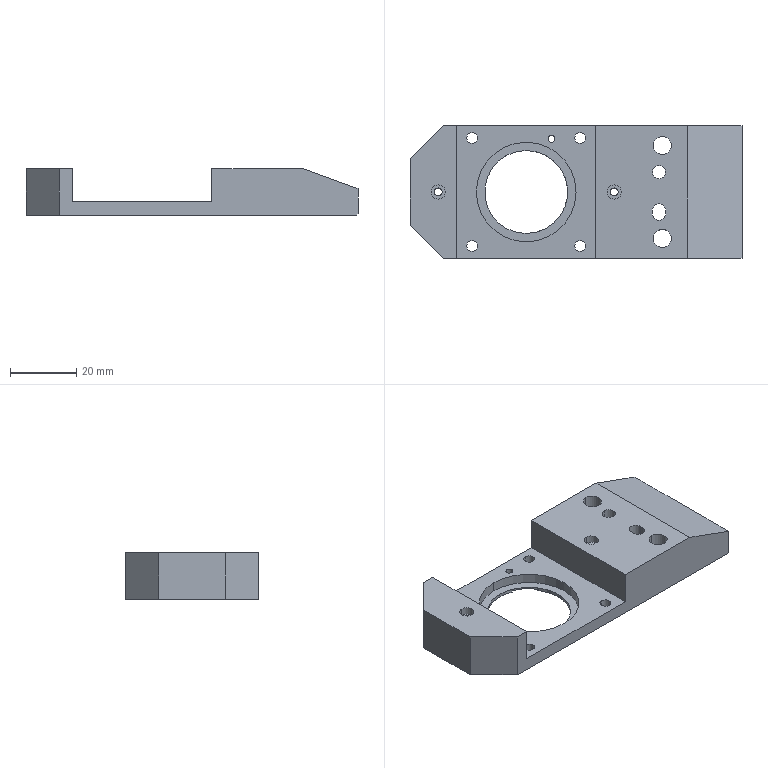NC program | NX | posted with a generic post | part box 100 x 40 x 14 mm
Whole program:
N10 G17 G21 G94 G90
(FLOOR_WALL_COPY_COPY , TOOL : D50R0.8)
N12 T03 M6
N14 G54
N16 G17 G0 G90 X-78.25 Y0. S1000 M3
N18 G43 Z30. H3
N20 Z8.707
N22 G94 G1 Z5.707 F1500.
N24 X-75.25
N26 X74.75
N28 X77.75
N30 Z8.707
N32 G0 Z30.
N34 X-78.25
N36 Z8.415
N38 G1 Z5.415
N40 X-75.25
N42 X74.75
N44 X77.75
N46 Z8.415
N48 G0 Z30.
N50 X-78.25
N52 Z8.122
N54 G1 Z5.122
N56 X-75.25
N58 X74.75
N60 X77.75
N62 Z8.122
N64 G0 Z30.
N66 X-78.25
N68 Z7.83
N70 G1 Z4.83
N72 X-75.25
N74 X74.75
N76 X77.75
N78 Z7.83
N80 G0 Z30.
N82 X-78.25
N84 Z7.537
N86 G1 Z4.537
N88 X-75.25
N90 X74.75
N92 X77.75
N94 Z7.537
N96 G0 Z30.
N98 X-78.25
N100 Z7.245
N102 G1 Z4.245
N104 X-75.25
N106 X74.75
N108 X77.75
N110 Z7.245
N112 G0 Z30.
N114 X-78.25
N116 Z6.952
N118 G1 Z3.952
N120 X-75.25
N122 X74.75
N124 X77.75
N126 Z6.952
N128 G0 Z30.
N130 X-78.25
N132 Z6.66
N134 G1 Z3.66
N136 X-75.25
N138 X74.75
N140 X77.75
N142 Z6.66
N144 G0 Z30.
N146 X-78.25
N148 Z6.367
N150 G1 Z3.367
N152 X-75.25
N154 X74.75
N156 X77.75
N158 Z6.367
N160 G0 Z30.
N162 X-78.25
N164 Z6.075
N166 G1 Z3.075
N168 X-75.25
N170 X74.75
N172 X77.75
N174 Z6.075
N176 G0 Z30.
N178 X-78.25
N180 Z5.782
N182 G1 Z2.782
N184 X-75.25
N186 X74.75
N188 X77.75
N190 Z5.782
N192 G0 Z30.
N194 X-78.25
N196 Z5.49
N198 G1 Z2.49
N200 X-75.25
N202 X74.75
N204 X77.75
N206 Z5.49
N208 G0 Z30.
N210 X-78.25
N212 Z5.197
N214 G1 Z2.197
N216 X-75.25
N218 X74.75
N220 X77.75
N222 Z5.197
N224 G0 Z30.
N226 X-78.25
N228 Z4.905
N230 G1 Z1.905
N232 X-75.25
N234 X74.75
N236 X77.75
N238 Z4.905
N240 G0 Z30.
N242 X-78.25
N244 Z4.612
N246 G1 Z1.612
N248 X-75.25
N250 X74.75
N252 X77.75
N254 Z4.612
N256 G0 Z30.
N258 X-78.25
N260 Z4.32
N262 G1 Z1.32
N264 X-75.25
N266 X74.75
N268 X77.75
N270 Z4.32
N272 G0 Z30.
N274 X-78.25
N276 Z4.027
N278 G1 Z1.027
N280 X-75.25
N282 X74.75
N284 X77.75
N286 Z4.027
N288 G0 Z30.
N290 X-78.25
N292 Z3.735
N294 G1 Z0.735
N296 X-75.25
N298 X74.75
N300 X77.75
N302 Z3.735
N304 G0 Z30.
N306 X-78.25
N308 Z3.442
N310 G1 Z0.442
N312 X-75.25
N314 X74.75
N316 X77.75
N318 Z3.442
N320 G0 Z30.
N322 X-78.25
N324 Z3.15
N326 G1 Z0.15
N328 X-75.25
N330 X74.75
N332 X77.75
N334 Z3.15
N336 G0 Z30.
(FLOOR_WALL_COPY_COPY_1 , TOOL : D50R0.8)
N338 X-78.25 S1500
N340 Z3.
N342 G1 Z0. F1000.
N344 X-75.25
N346 X74.75
N348 X77.75
N350 Z3.
N352 G0 Z30.
N354 M5
(HOLE_MILLING_1 , TOOL : D6)
N356 T06 M6
N358 G54
N360 G17 G0 G90 X-26.25 Y14. S4000 M3
N362 G43 Z30. H6
N364 Z0.5
N366 G94 G3 X-27.225 Y14.975 R0.975 F1800.
N368 X-28.2 Y14. R0.975
N370 X-28.2 Y14. Z0.4 I1.95 J0.
N372 X-28.2 Y14. Z0.3 I1.95 J0.
N374 X-28.2 Y14. Z0.2 I1.95 J0.
N376 X-28.2 Y14. Z0.1 I1.95 J0.
N378 X-28.2 Y14. Z0. I1.95 J0.
N380 X-28.2 Y14. Z-0.1 I1.95 J0.
N382 X-28.2 Y14. Z-0.2 I1.95 J0.
N384 X-28.2 Y14. Z-0.3 I1.95 J0.
N386 X-28.2 Y14. Z-0.4 I1.95 J0.
N388 X-28.2 Y14. Z-0.5 I1.95 J0.
N390 X-28.2 Y14. Z-0.6 I1.95 J0.
N392 X-28.2 Y14. Z-0.7 I1.95 J0.
N394 X-28.2 Y14. Z-0.8 I1.95 J0.
N396 X-28.2 Y14. Z-0.9 I1.95 J0.
N398 X-28.2 Y14. Z-1. I1.95 J0.
N400 X-28.2 Y14. Z-1.1 I1.95 J0.
N402 X-28.2 Y14. Z-1.2 I1.95 J0.
N404 X-28.2 Y14. Z-1.3 I1.95 J0.
N406 X-28.2 Y14. Z-1.4 I1.95 J0.
N408 X-28.2 Y14. Z-1.5 I1.95 J0.
N410 X-28.2 Y14. Z-1.6 I1.95 J0.
N412 X-28.2 Y14. Z-1.7 I1.95 J0.
N414 X-28.2 Y14. Z-1.8 I1.95 J0.
N416 X-28.2 Y14. Z-1.9 I1.95 J0.
N418 X-28.2 Y14. Z-2. I1.95 J0.
N420 X-28.2 Y14. Z-2.1 I1.95 J0.
N422 X-28.2 Y14. Z-2.2 I1.95 J0.
N424 X-28.2 Y14. Z-2.3 I1.95 J0.
N426 X-28.2 Y14. Z-2.4 I1.95 J0.
N428 X-28.2 Y14. Z-2.5 I1.95 J0.
N430 X-28.2 Y14. Z-2.6 I1.95 J0.
N432 X-28.2 Y14. Z-2.7 I1.95 J0.
N434 X-28.2 Y14. Z-2.8 I1.95 J0.
N436 X-28.2 Y14. Z-2.9 I1.95 J0.
N438 X-28.2 Y14. Z-3. I1.95 J0.
N440 X-28.2 Y14. Z-3.1 I1.95 J0.
N442 X-28.2 Y14. Z-3.2 I1.95 J0.
N444 X-28.2 Y14. Z-3.3 I1.95 J0.
N446 X-28.2 Y14. Z-3.4 I1.95 J0.
N448 X-28.2 Y14. Z-3.5 I1.95 J0.
N450 X-28.2 Y14. Z-3.6 I1.95 J0.
N452 X-28.2 Y14. Z-3.7 I1.95 J0.
N454 X-28.2 Y14. Z-3.8 I1.95 J0.
N456 X-28.2 Y14. Z-3.9 I1.95 J0.
N458 X-28.2 Y14. Z-4. I1.95 J0.
N460 X-28.2 Y14. Z-4.1 I1.95 J0.
N462 X-28.2 Y14. Z-4.2 I1.95 J0.
N464 X-28.2 Y14. Z-4.3 I1.95 J0.
N466 X-28.2 Y14. Z-4.4 I1.95 J0.
N468 X-28.2 Y14. Z-4.5 I1.95 J0.
N470 X-28.2 Y14. Z-4.6 I1.95 J0.
N472 X-28.2 Y14. Z-4.7 I1.95 J0.
N474 X-28.2 Y14. Z-4.8 I1.95 J0.
N476 X-28.2 Y14. Z-4.9 I1.95 J0.
N478 X-28.2 Y14. Z-5. I1.95 J0.
N480 X-28.2 Y14. Z-5.1 I1.95 J0.
N482 X-28.2 Y14. Z-5.2 I1.95 J0.
N484 X-28.2 Y14. Z-5.3 I1.95 J0.
N486 X-28.2 Y14. Z-5.4 I1.95 J0.
N488 X-28.2 Y14. Z-5.5 I1.95 J0.
N490 X-28.2 Y14. Z-5.6 I1.95 J0.
N492 X-28.2 Y14. Z-5.7 I1.95 J0.
N494 X-26.25 Y12.05 R1.95
N496 X-28.2 Y14. R-1.95
N498 X-27.225 Y13.025 R0.975
N500 X-26.25 Y14. R0.975
N502 G0 Z30.
N504 Y-14.
N506 Z0.5
N508 G3 X-27.225 Y-13.025 R0.975
N510 X-28.2 Y-14. R0.975
N512 X-28.2 Y-14. Z0.4 I1.95 J0.
N514 X-28.2 Y-14. Z0.3 I1.95 J0.
N516 X-28.2 Y-14. Z0.2 I1.95 J0.
N518 X-28.2 Y-14. Z0.1 I1.95 J0.
N520 X-28.2 Y-14. Z0. I1.95 J0.
N522 X-28.2 Y-14. Z-0.1 I1.95 J0.
N524 X-28.2 Y-14. Z-0.2 I1.95 J0.
N526 X-28.2 Y-14. Z-0.3 I1.95 J0.
N528 X-28.2 Y-14. Z-0.4 I1.95 J0.
N530 X-28.2 Y-14. Z-0.5 I1.95 J0.
N532 X-28.2 Y-14. Z-0.6 I1.95 J0.
N534 X-28.2 Y-14. Z-0.7 I1.95 J0.
N536 X-28.2 Y-14. Z-0.8 I1.95 J0.
N538 X-28.2 Y-14. Z-0.9 I1.95 J0.
N540 X-28.2 Y-14. Z-1. I1.95 J0.
N542 X-28.2 Y-14. Z-1.1 I1.95 J0.
N544 X-28.2 Y-14. Z-1.2 I1.95 J0.
N546 X-28.2 Y-14. Z-1.3 I1.95 J0.
N548 X-28.2 Y-14. Z-1.4 I1.95 J0.
N550 X-28.2 Y-14. Z-1.5 I1.95 J0.
N552 X-28.2 Y-14. Z-1.6 I1.95 J0.
N554 X-28.2 Y-14. Z-1.7 I1.95 J0.
N556 X-28.2 Y-14. Z-1.8 I1.95 J0.
N558 X-28.2 Y-14. Z-1.9 I1.95 J0.
N560 X-28.2 Y-14. Z-2. I1.95 J0.
N562 X-28.2 Y-14. Z-2.1 I1.95 J0.
N564 X-28.2 Y-14. Z-2.2 I1.95 J0.
N566 X-28.2 Y-14. Z-2.3 I1.95 J0.
N568 X-28.2 Y-14. Z-2.4 I1.95 J0.
N570 X-28.2 Y-14. Z-2.5 I1.95 J0.
N572 X-28.2 Y-14. Z-2.6 I1.95 J0.
N574 X-28.2 Y-14. Z-2.7 I1.95 J0.
N576 X-28.2 Y-14. Z-2.8 I1.95 J0.
N578 X-28.2 Y-14. Z-2.9 I1.95 J0.
N580 X-28.2 Y-14. Z-3. I1.95 J0.
N582 X-28.2 Y-14. Z-3.1 I1.95 J0.
N584 X-28.2 Y-14. Z-3.2 I1.95 J0.
N586 X-28.2 Y-14. Z-3.3 I1.95 J0.
N588 X-28.2 Y-14. Z-3.4 I1.95 J0.
N590 X-28.2 Y-14. Z-3.5 I1.95 J0.
N592 X-28.2 Y-14. Z-3.6 I1.95 J0.
N594 X-28.2 Y-14. Z-3.7 I1.95 J0.
N596 X-28.2 Y-14. Z-3.8 I1.95 J0.
N598 X-28.2 Y-14. Z-3.9 I1.95 J0.
N600 X-28.2 Y-14. Z-4. I1.95 J0.
N602 X-28.2 Y-14. Z-4.1 I1.95 J0.
N604 X-28.2 Y-14. Z-4.2 I1.95 J0.
N606 X-28.2 Y-14. Z-4.3 I1.95 J0.
N608 X-28.2 Y-14. Z-4.4 I1.95 J0.
N610 X-28.2 Y-14. Z-4.5 I1.95 J0.
N612 X-28.2 Y-14. Z-4.6 I1.95 J0.
N614 X-28.2 Y-14. Z-4.7 I1.95 J0.
N616 X-28.2 Y-14. Z-4.8 I1.95 J0.
N618 X-28.2 Y-14. Z-4.9 I1.95 J0.
N620 X-28.2 Y-14. Z-5. I1.95 J0.
N622 X-28.2 Y-14. Z-5.1 I1.95 J0.
N624 X-28.2 Y-14. Z-5.2 I1.95 J0.
N626 X-28.2 Y-14. Z-5.3 I1.95 J0.
N628 X-28.2 Y-14. Z-5.4 I1.95 J0.
N630 X-28.2 Y-14. Z-5.5 I1.95 J0.
N632 X-28.2 Y-14. Z-5.6 I1.95 J0.
N634 X-28.2 Y-14. Z-5.7 I1.95 J0.
N636 X-26.25 Y-15.95 R1.95
N638 X-28.2 Y-14. R-1.95
N640 X-27.225 Y-14.975 R0.975
N642 X-26.25 Y-14. R0.975
N644 G0 Z30.
N646 X-11.75 Y0.
N648 Z0.5
N650 G3 X-11.975 Y0.225 R0.225
N652 X-12.2 Y0. R0.225
N654 X-12.2 Y0. Z0.4 I0.45 J0.
N656 X-12.2 Y0. Z0.3 I0.45 J0.
N658 X-12.2 Y0. Z0.2 I0.45 J0.
N660 X-12.2 Y0. Z0.1 I0.45 J0.
N662 X-12.2 Y0. Z0. I0.45 J0.
N664 X-12.2 Y0. Z-0.1 I0.45 J0.
N666 X-12.2 Y0. Z-0.2 I0.45 J0.
N668 X-12.2 Y0. Z-0.3 I0.45 J0.
N670 X-12.2 Y0. Z-0.4 I0.45 J0.
N672 X-12.2 Y0. Z-0.5 I0.45 J0.
N674 X-12.2 Y0. Z-0.6 I0.45 J0.
N676 X-12.2 Y0. Z-0.7 I0.45 J0.
N678 X-12.2 Y0. Z-0.8 I0.45 J0.
N680 X-12.2 Y0. Z-0.9 I0.45 J0.
N682 X-12.2 Y0. Z-1. I0.45 J0.
N684 X-12.2 Y0. Z-1.1 I0.45 J0.
N686 X-12.2 Y0. Z-1.2 I0.45 J0.
N688 X-12.2 Y0. Z-1.3 I0.45 J0.
N690 X-12.2 Y0. Z-1.4 I0.45 J0.
N692 X-12.2 Y0. Z-1.5 I0.45 J0.
N694 X-12.2 Y0. Z-1.6 I0.45 J0.
N696 X-12.2 Y0. Z-1.7 I0.45 J0.
N698 X-12.2 Y0. Z-1.8 I0.45 J0.
N700 X-12.2 Y0. Z-1.9 I0.45 J0.
N702 X-12.2 Y0. Z-2. I0.45 J0.
N704 X-12.2 Y0. Z-2.1 I0.45 J0.
N706 X-12.2 Y0. Z-2.2 I0.45 J0.
N708 X-12.2 Y0. Z-2.3 I0.45 J0.
N710 X-12.2 Y0. Z-2.4 I0.45 J0.
N712 X-12.2 Y0. Z-2.5 I0.45 J0.
N714 X-12.2 Y0. Z-2.6 I0.45 J0.
N716 X-12.2 Y0. Z-2.7 I0.45 J0.
N718 X-12.2 Y0. Z-2.8 I0.45 J0.
N720 X-12.2 Y0. Z-2.9 I0.45 J0.
N722 X-12.2 Y0. Z-3. I0.45 J0.
N724 X-12.2 Y0. Z-3.1 I0.45 J0.
N726 X-12.2 Y0. Z-3.2 I0.45 J0.
N728 X-12.2 Y0. Z-3.3 I0.45 J0.
N730 X-12.2 Y0. Z-3.4 I0.45 J0.
N732 X-12.2 Y0. Z-3.5 I0.45 J0.
N734 X-12.2 Y0. Z-3.6 I0.45 J0.
N736 X-12.2 Y0. Z-3.7 I0.45 J0.
N738 X-12.2 Y0. Z-3.8 I0.45 J0.
N740 X-12.2 Y0. Z-3.9 I0.45 J0.
N742 X-12.2 Y0. Z-4. I0.45 J0.
N744 X-12.2 Y0. Z-4.1 I0.45 J0.
N746 X-12.2 Y0. Z-4.2 I0.45 J0.
N748 X-12.2 Y0. Z-4.3 I0.45 J0.
N750 X-12.2 Y0. Z-4.4 I0.45 J0.
N752 X-12.2 Y0. Z-4.5 I0.45 J0.
N754 X-12.2 Y0. Z-4.6 I0.45 J0.
N756 X-12.2 Y0. Z-4.7 I0.45 J0.
N758 X-12.2 Y0. Z-4.8 I0.45 J0.
N760 X-12.2 Y0. Z-4.9 I0.45 J0.
N762 X-12.2 Y0. Z-5. I0.45 J0.
N764 X-12.2 Y0. Z-5.1 I0.45 J0.
N766 X-12.2 Y0. Z-5.2 I0.45 J0.
N768 X-12.2 Y0. Z-5.3 I0.45 J0.
N770 X-12.2 Y0. Z-5.4 I0.45 J0.
N772 X-12.2 Y0. Z-5.5 I0.45 J0.
N774 X-12.2 Y0. Z-5.6 I0.45 J0.
N776 X-12.2 Y0. Z-5.7 I0.45 J0.
N778 X-12.2 Y0. Z-5.8 I0.45 J0.
N780 X-12.2 Y0. Z-5.9 I0.45 J0.
N782 X-12.2 Y0. Z-6. I0.45 J0.
N784 X-11.75 Y-0.45 R0.45
N786 X-12.2 Y0. R-0.45
N788 X-11.975 Y-0.225 R0.225
N790 X-11.75 Y0. R0.225
N792 G0 Z30.
N794 X41.25
N796 Z0.5
N798 G3 X41.025 Y0.225 R0.225
N800 X40.8 Y0. R0.225
N802 X40.8 Y0. Z0.4 I0.45 J0.
N804 X40.8 Y0. Z0.3 I0.45 J0.
N806 X40.8 Y0. Z0.2 I0.45 J0.
N808 X40.8 Y0. Z0.1 I0.45 J0.
N810 X40.8 Y0. Z0. I0.45 J0.
N812 X40.8 Y0. Z-0.1 I0.45 J0.
N814 X40.8 Y0. Z-0.2 I0.45 J0.
N816 X40.8 Y0. Z-0.3 I0.45 J0.
N818 X40.8 Y0. Z-0.4 I0.45 J0.
N820 X40.8 Y0. Z-0.5 I0.45 J0.
N822 X40.8 Y0. Z-0.6 I0.45 J0.
N824 X40.8 Y0. Z-0.7 I0.45 J0.
N826 X40.8 Y0. Z-0.8 I0.45 J0.
N828 X40.8 Y0. Z-0.9 I0.45 J0.
N830 X40.8 Y0. Z-1. I0.45 J0.
N832 X40.8 Y0. Z-1.1 I0.45 J0.
N834 X40.8 Y0. Z-1.2 I0.45 J0.
N836 X40.8 Y0. Z-1.3 I0.45 J0.
N838 X40.8 Y0. Z-1.4 I0.45 J0.
N840 X40.8 Y0. Z-1.5 I0.45 J0.
N842 X40.8 Y0. Z-1.6 I0.45 J0.
N844 X40.8 Y0. Z-1.7 I0.45 J0.
N846 X40.8 Y0. Z-1.8 I0.45 J0.
N848 X40.8 Y0. Z-1.9 I0.45 J0.
N850 X40.8 Y0. Z-2. I0.45 J0.
N852 X40.8 Y0. Z-2.1 I0.45 J0.
N854 X40.8 Y0. Z-2.2 I0.45 J0.
N856 X40.8 Y0. Z-2.3 I0.45 J0.
N858 X40.8 Y0. Z-2.4 I0.45 J0.
N860 X40.8 Y0. Z-2.5 I0.45 J0.
N862 X40.8 Y0. Z-2.6 I0.45 J0.
N864 X40.8 Y0. Z-2.7 I0.45 J0.
N866 X40.8 Y0. Z-2.8 I0.45 J0.
N868 X40.8 Y0. Z-2.9 I0.45 J0.
N870 X40.8 Y0. Z-3. I0.45 J0.
N872 X40.8 Y0. Z-3.1 I0.45 J0.
N874 X40.8 Y0. Z-3.2 I0.45 J0.
N876 X40.8 Y0. Z-3.3 I0.45 J0.
N878 X40.8 Y0. Z-3.4 I0.45 J0.
N880 X40.8 Y0. Z-3.5 I0.45 J0.
N882 X40.8 Y0. Z-3.6 I0.45 J0.
N884 X40.8 Y0. Z-3.7 I0.45 J0.
N886 X40.8 Y0. Z-3.8 I0.45 J0.
N888 X40.8 Y0. Z-3.9 I0.45 J0.
N890 X40.8 Y0. Z-4. I0.45 J0.
N892 X40.8 Y0. Z-4.1 I0.45 J0.
N894 X40.8 Y0. Z-4.2 I0.45 J0.
N896 X40.8 Y0. Z-4.3 I0.45 J0.
N898 X40.8 Y0. Z-4.4 I0.45 J0.
N900 X40.8 Y0. Z-4.5 I0.45 J0.
N902 X40.8 Y0. Z-4.6 I0.45 J0.
N904 X40.8 Y0. Z-4.7 I0.45 J0.
N906 X40.8 Y0. Z-4.8 I0.45 J0.
N908 X40.8 Y0. Z-4.9 I0.45 J0.
N910 X40.8 Y0. Z-5. I0.45 J0.
N912 X40.8 Y0. Z-5.1 I0.45 J0.
N914 X40.8 Y0. Z-5.2 I0.45 J0.
N916 X40.8 Y0. Z-5.3 I0.45 J0.
N918 X40.8 Y0. Z-5.4 I0.45 J0.
N920 X40.8 Y0. Z-5.5 I0.45 J0.
N922 X40.8 Y0. Z-5.6 I0.45 J0.
N924 X40.8 Y0. Z-5.7 I0.45 J0.
N926 X40.8 Y0. Z-5.8 I0.45 J0.
N928 X40.8 Y0. Z-5.9 I0.45 J0.
N930 X40.8 Y0. Z-6. I0.45 J0.
N932 X41.25 Y-0.45 R0.45
N934 X40.8 Y0. R-0.45
N936 X41.025 Y-0.225 R0.225
N938 X41.25 Y0. R0.225
N940 G0 Z30.
N942 M5
(HOLE_MILLING_1_COPY , TOOL : D6JING)
N944 T16 M6
N946 G54
N948 G17 G0 G90 X-26.25 Y14. S5500 M3
N950 G43 Z30. H16
N952 Z0.5
N954 G94 G3 X-27.25 Y15. R1. F1000.
N956 X-28.25 Y14. R1.
N958 X-28.25 Y14. Z-1.5 I2. J0.
N960 X-28.25 Y14. Z-3.5 I2. J0.
N962 X-28.25 Y14. Z-5.5 I2. J0.
N964 X-27.868 Y12.824 Z-5.7 R2.
N966 X-25.074 Y12.382 R2.
N968 X-27.868 Y12.824 R-2.
N970 X-26.471 Y12.603 R1.
N972 X-26.25 Y14. R1.
N974 G0 Z30.
N976 Y-14.
N978 Z0.5
N980 G3 X-27.25 Y-13. R1.
N982 X-28.25 Y-14. R1.
N984 X-28.25 Y-14. Z-1.5 I2. J0.
N986 X-28.25 Y-14. Z-3.5 I2. J0.
N988 X-28.25 Y-14. Z-5.5 I2. J0.
N990 X-27.868 Y-15.176 Z-5.7 R2.
N992 X-25.074 Y-15.618 R2.
N994 X-27.868 Y-15.176 R-2.
N996 X-26.471 Y-15.397 R1.
N998 X-26.25 Y-14. R1.
N1000 G0 Z30.
N1002 X-11.75 Y0.
N1004 Z0.5
N1006 G3 X-12. Y0.25 R0.25
N1008 X-12.25 Y0. R0.25
N1010 X-12.25 Y0. Z-1.5 I0.5 J0.
N1012 X-12.25 Y0. Z-3.5 I0.5 J0.
N1014 X-12.25 Y0. Z-5.5 I0.5 J0.
N1016 X-11.75 Y-0.5 Z-6. R0.5
N1018 X-11.25 Y0. R0.5
N1020 X-11.75 Y-0.5 R-0.5
N1022 X-11.5 Y-0.25 R0.25
N1024 X-11.75 Y0. R0.25
N1026 G0 Z30.
N1028 X41.25
N1030 Z0.5
N1032 G3 X41. Y0.25 R0.25
N1034 X40.75 Y0. R0.25
N1036 X40.75 Y0. Z-1.5 I0.5 J0.
N1038 X40.75 Y0. Z-3.5 I0.5 J0.
N1040 X40.75 Y0. Z-5.5 I0.5 J0.
N1042 X41.25 Y-0.5 Z-6. R0.5
N1044 X41.75 Y0. R0.5
N1046 X41.25 Y-0.5 R-0.5
N1048 X41.5 Y-0.25 R0.25
N1050 X41.25 Y0. R0.25
N1052 G0 Z30.
(FLOOR_WALL_COPY_1 , TOOL : D6JING)
N1054 X7.569 Y4.552 S6500
N1056 Z0.875
N1058 G1 Z-0.125 F1250.
N1060 X6.751 Y5.046
N1062 G3 X7.051 Y5.566 R0.6
N1064 G1 Y23.
N1066 X7.25
N1068 Y5.831
N1070 G2 X6.95 Y5.311 R0.6
N1072 G1 X7.724 Y4.784
N1074 Z0.875
N1076 G0 Z30.
N1078 X7.569 Y4.552
N1080 Z0.75
N1082 G1 Z-0.25
N1084 X6.751 Y5.046
N1086 G3 X7.051 Y5.566 R0.6
N1088 G1 Y23.
N1090 X7.25
N1092 Y5.831
N1094 G2 X6.95 Y5.311 R0.6
N1096 G1 X7.724 Y4.784
N1098 Z0.75
N1100 G0 Z30.
N1102 X7.569 Y4.552
N1104 Z0.625
N1106 G1 Z-0.375
N1108 X6.751 Y5.046
N1110 G3 X7.051 Y5.566 R0.6
N1112 G1 Y23.
N1114 X7.25
N1116 Y5.831
N1118 G2 X6.95 Y5.311 R0.6
N1120 G1 X7.724 Y4.784
N1122 Z0.625
N1124 G0 Z30.
N1126 X7.569 Y4.552
N1128 Z0.5
N1130 G1 Z-0.5
N1132 X6.751 Y5.046
N1134 G3 X7.051 Y5.566 R0.6
N1136 G1 Y23.
N1138 X7.25
N1140 Y5.831
N1142 G2 X6.95 Y5.311 R0.6
N1144 G1 X7.724 Y4.784
N1146 Z0.5
N1148 G0 Z30.
N1150 M5
(HOLE_MILLING_COPY , TOOL : D3)
N1152 T17 M6
N1154 G54
N1156 G17 G0 G90 X-11.75 Y0. S5500 M3
N1158 G43 Z30. H17
N1160 Z-5.5
N1162 G94 G3 X-11.975 Y0.225 R0.225 F1250.
N1164 X-12.2 Y0. R0.225
N1166 X-12.2 Y0. Z-5.56 I0.45 J0.
N1168 X-12.2 Y0. Z-5.62 I0.45 J0.
N1170 X-12.2 Y0. Z-5.68 I0.45 J0.
N1172 X-12.2 Y0. Z-5.74 I0.45 J0.
N1174 X-12.2 Y0. Z-5.8 I0.45 J0.
N1176 X-12.2 Y0. Z-5.86 I0.45 J0.
N1178 X-12.2 Y0. Z-5.92 I0.45 J0.
N1180 X-12.2 Y0. Z-5.98 I0.45 J0.
N1182 X-12.2 Y0. Z-6.04 I0.45 J0.
N1184 X-12.2 Y0. Z-6.1 I0.45 J0.
N1186 X-12.2 Y0. Z-6.16 I0.45 J0.
N1188 X-12.2 Y0. Z-6.22 I0.45 J0.
N1190 X-12.2 Y0. Z-6.28 I0.45 J0.
N1192 X-12.2 Y0. Z-6.34 I0.45 J0.
N1194 X-12.2 Y0. Z-6.4 I0.45 J0.
N1196 X-12.2 Y0. Z-6.46 I0.45 J0.
N1198 X-12.2 Y0. Z-6.52 I0.45 J0.
N1200 X-12.2 Y0. Z-6.58 I0.45 J0.
N1202 X-12.2 Y0. Z-6.64 I0.45 J0.
N1204 X-12.2 Y0. Z-6.7 I0.45 J0.
N1206 X-12.2 Y0. Z-6.76 I0.45 J0.
N1208 X-12.2 Y0. Z-6.82 I0.45 J0.
N1210 X-12.2 Y0. Z-6.88 I0.45 J0.
N1212 X-12.2 Y0. Z-6.94 I0.45 J0.
N1214 X-12.2 Y0. Z-7. I0.45 J0.
N1216 X-12.2 Y0. Z-7.06 I0.45 J0.
N1218 X-12.2 Y0. Z-7.12 I0.45 J0.
N1220 X-12.2 Y0. Z-7.18 I0.45 J0.
N1222 X-12.2 Y0. Z-7.24 I0.45 J0.
N1224 X-12.2 Y0. Z-7.3 I0.45 J0.
N1226 X-12.2 Y0. Z-7.36 I0.45 J0.
N1228 X-12.2 Y0. Z-7.42 I0.45 J0.
N1230 X-12.2 Y0. Z-7.48 I0.45 J0.
N1232 X-12.2 Y0. Z-7.54 I0.45 J0.
N1234 X-12.2 Y0. Z-7.6 I0.45 J0.
N1236 X-12.2 Y0. Z-7.66 I0.45 J0.
N1238 X-12.2 Y0. Z-7.72 I0.45 J0.
N1240 X-12.2 Y0. Z-7.78 I0.45 J0.
N1242 X-12.2 Y0. Z-7.84 I0.45 J0.
N1244 X-12.2 Y0. Z-7.9 I0.45 J0.
N1246 X-12.2 Y0. Z-7.96 I0.45 J0.
N1248 X-12.2 Y0. Z-8.02 I0.45 J0.
N1250 X-12.2 Y0. Z-8.08 I0.45 J0.
N1252 X-12.2 Y0. Z-8.14 I0.45 J0.
N1254 X-12.2 Y0. Z-8.2 I0.45 J0.
N1256 X-12.2 Y0. Z-8.26 I0.45 J0.
N1258 X-11.525 Y0.39 Z-8.3 R-0.45
N1260 X-12.14 Y0.225 R0.45
N1262 X-11.525 Y0.39 R-0.45
N1264 X-11.832 Y0.307 R0.225
N1266 X-11.75 Y0. R0.225
N1268 G0 Z30.
N1270 X41.25
N1272 Z-5.5
N1274 G3 X41.025 Y0.225 R0.225
N1276 X40.8 Y0. R0.225
N1278 X40.8 Y0. Z-5.56 I0.45 J0.
N1280 X40.8 Y0. Z-5.62 I0.45 J0.
N1282 X40.8 Y0. Z-5.68 I0.45 J0.
N1284 X40.8 Y0. Z-5.74 I0.45 J0.
N1286 X40.8 Y0. Z-5.8 I0.45 J0.
N1288 X40.8 Y0. Z-5.86 I0.45 J0.
N1290 X40.8 Y0. Z-5.92 I0.45 J0.
N1292 X40.8 Y0. Z-5.98 I0.45 J0.
N1294 X40.8 Y0. Z-6.04 I0.45 J0.
N1296 X40.8 Y0. Z-6.1 I0.45 J0.
N1298 X40.8 Y0. Z-6.16 I0.45 J0.
N1300 X40.8 Y0. Z-6.22 I0.45 J0.
N1302 X40.8 Y0. Z-6.28 I0.45 J0.
N1304 X40.8 Y0. Z-6.34 I0.45 J0.
N1306 X40.8 Y0. Z-6.4 I0.45 J0.
N1308 X40.8 Y0. Z-6.46 I0.45 J0.
N1310 X40.8 Y0. Z-6.52 I0.45 J0.
N1312 X40.8 Y0. Z-6.58 I0.45 J0.
N1314 X40.8 Y0. Z-6.64 I0.45 J0.
N1316 X40.8 Y0. Z-6.7 I0.45 J0.
N1318 X40.8 Y0. Z-6.76 I0.45 J0.
N1320 X40.8 Y0. Z-6.82 I0.45 J0.
N1322 X40.8 Y0. Z-6.88 I0.45 J0.
N1324 X40.8 Y0. Z-6.94 I0.45 J0.
N1326 X40.8 Y0. Z-7. I0.45 J0.
N1328 X40.8 Y0. Z-7.06 I0.45 J0.
N1330 X40.8 Y0. Z-7.12 I0.45 J0.
N1332 X40.8 Y0. Z-7.18 I0.45 J0.
N1334 X40.8 Y0. Z-7.24 I0.45 J0.
N1336 X40.8 Y0. Z-7.3 I0.45 J0.
N1338 X40.8 Y0. Z-7.36 I0.45 J0.
N1340 X40.8 Y0. Z-7.42 I0.45 J0.
N1342 X40.8 Y0. Z-7.48 I0.45 J0.
N1344 X40.8 Y0. Z-7.54 I0.45 J0.
N1346 X40.8 Y0. Z-7.6 I0.45 J0.
N1348 X40.8 Y0. Z-7.66 I0.45 J0.
N1350 X40.8 Y0. Z-7.72 I0.45 J0.
N1352 X40.8 Y0. Z-7.78 I0.45 J0.
N1354 X40.8 Y0. Z-7.84 I0.45 J0.
N1356 X40.8 Y0. Z-7.9 I0.45 J0.
N1358 X40.8 Y0. Z-7.96 I0.45 J0.
N1360 X40.8 Y0. Z-8.02 I0.45 J0.
N1362 X40.8 Y0. Z-8.08 I0.45 J0.
N1364 X40.8 Y0. Z-8.14 I0.45 J0.
N1366 X40.8 Y0. Z-8.2 I0.45 J0.
N1368 X40.8 Y0. Z-8.26 I0.45 J0.
N1370 X41.475 Y0.39 Z-8.3 R-0.45
N1372 X40.86 Y0.225 R0.45
N1374 X41.475 Y0.39 R-0.45
N1376 X41.168 Y0.307 R0.225
N1378 X41.25 Y0. R0.225
N1380 G0 Z30.
N1382 M5
(11_COPY_COPY_COPY_COPY_COPY_1 , TOOL : D6A45)
N1384 T01 M6
N1386 G54
N1388 G17 G0 G90 X-1.513 Y16.957 S7500 M3
N1390 G43 Z30. H1
N1392 Z3.
N1394 G94 G1 Z-1. F1000.
N1396 X-1.517
N1398 G3 X-2.207 Y16.26 R0.694
N1400 X-1.513 Y16.957 R-0.694
N1402 X-2.033 Y16.657 R0.6
N1404 G1 Z2.
N1406 G0 Z30.
N1408 X-25.06 Y16.583
N1410 Z2.
N1412 G1 Z-1.
N1414 X-25.73 Y17.744
N1416 G3 X-26.25 Y18.044 R0.6
N1418 G1 X-26.255
N1420 G3 X-30.294 Y13.995 R4.044
N1422 X-26.25 Y18.044 R-4.044
N1424 X-26.77 Y17.744 R0.6
N1426 G1 X-27.44 Y16.583
N1428 Z2.
N1430 G0 Z30.
N1432 X-25.25 Y7.044
N1434 Z3.
N1436 G1 Z-1.
N1438 G3 X-26.294 Y6. R1.044
N1440 X-25.25 Y7.044 R-1.044
N1442 X-25.77 Y6.744 R0.6
N1444 G1 Z2.
N1446 G0 Z30.
N1448 X42.559 Y-0.303
N1450 Z2.
N1452 G1 Z-1.
N1454 X43.494 Y-0.52
N1456 G3 X43.794 Y0. R0.6
N1458 X41.25 Y2.544 R2.544
N1460 X43.794 Y0. R-2.544
N1462 X43.494 Y0.52 R0.6
N1464 G1 X42.559 Y0.303
N1466 Z2.
N1468 G0 Z30.
N1470 X-11.447 Y1.309
N1472 Z2.
N1474 G1 Z-1.
N1476 X-11.23 Y2.244
N1478 G3 X-11.75 Y2.544 R0.6
N1480 G1 X-11.753
N1482 G3 X-14.294 Y-0.003 R2.544
N1484 X-11.75 Y2.544 R-2.544
N1486 X-12.27 Y2.244 R0.6
N1488 G1 X-12.053 Y1.309
N1490 Z2.
N1492 G0 Z30.
N1494 X-26.294 Y-5.5
N1496 Z3.
N1498 G1 Z-1.
N1500 Y-6.5
N1502 G3 X-25.25 Y-7.544 R1.044
N1504 X-24.206 Y-6.5 R1.044
N1506 G1 Y-5.5
N1508 G3 X-25.25 Y-4.456 R1.044
N1510 X-26.294 Y-5.5 R1.044
N1512 X-25.994 Y-6.02 R0.6
N1514 G1 Z2.
N1516 G0 Z30.
N1518 X31.013 Y16.957
N1520 Z3.
N1522 G1 Z-1.
N1524 X31.009
N1526 G3 X30.32 Y16.259 R0.694
N1528 X31.013 Y16.957 R-0.694
N1530 X30.494 Y16.657 R0.6
N1532 G1 Z2.
N1534 G0 Z30.
N1536 X6.195 Y6.242
N1538 Z2.
N1540 G1 Z-1.
N1542 X5.394 Y6.258
N1544 G3 X4.869 Y5.968 R0.6
N1546 X10.594 Y10.77 R-11.544
N1548 G2 X9.657 Y10.914 R0.95
N1550 G3 X5.006 Y7.079 R12.044
N1552 G1 Y6.461
N1554 G2 X4.869 Y5.968 R0.953
N1556 G3 X4.857 Y5.369 R0.6
N1558 G1 X5.39 Y4.402
N1560 Z2.
N1562 G0 Z30.
N1564 X31.013 Y-16.957
N1566 Z3.
N1568 G1 Z-1.
N1570 G3 X31.707 Y-16.263 R0.694
N1572 X31.013 Y-16.957 R-0.694
N1574 X31.533 Y-16.657 R0.6
N1576 G1 Z2.
N1578 G0 Z30.
N1580 X-1.513 Y-16.957
N1582 Z3.
N1584 G1 Z-1.
N1586 G3 X-0.82 Y-16.263 R0.694
N1588 X-1.513 Y-16.957 R-0.694
N1590 X-0.994 Y-16.657 R0.6
N1592 G1 Z2.
N1594 G0 Z30.
N1596 X-27.44 Y-16.583
N1598 Z2.
N1600 G1 Z-1.
N1602 X-26.77 Y-17.744
N1604 G3 X-26.25 Y-18.044 R0.6
N1606 X-22.206 Y-14. R4.044
N1608 X-26.25 Y-18.044 R-4.044
N1610 X-25.73 Y-17.744 R0.6
N1612 G1 X-25.06 Y-16.583
N1614 Z2.
N1616 G0 Z30.
N1618 X7.15 Y16.569
N1620 Z3.
N1622 G1 Z-1.
N1624 G3 X6.581 Y16. R0.569
N1626 X7.15 Y16.569 R-0.569
N1628 X6.89 Y16.419 R0.3
N1630 G1 Z2.
N1632 G0 Z30.
N1634 X40.671 Y-21.95
N1636 Z2.
N1638 G1 Z-1.
N1640 X40.27 Y-21.256
N1642 G3 X39.751 Y-20.956 R0.6
N1644 G1 X-49.751
N1646 G2 X-50.706 Y-20.001 R0.955
N1648 G1 Y20.001
N1650 G2 X-49.751 Y20.956 R0.955
N1652 G1 X4.051
N1654 G2 X4.89 Y20.456 R0.971
N1656 G1 X9.411
N1658 G2 X10.246 Y20.956 R0.962
N1660 G1 X39.751
N1662 G2 X40.426 Y20.677 R0.954
N1664 G1 X50.427 Y10.675
N1666 G2 X50.706 Y10.001 R0.954
N1668 G1 Y-10.001
N1670 G2 X50.427 Y-10.675 R0.954
N1672 G1 X40.426 Y-20.677
N1674 G2 X39.751 Y-20.956 R0.954
N1676 G3 X39.231 Y-21.256 R0.6
N1678 G1 X38.711 Y-22.156
N1680 Z2.
N1682 G0 Z30.
N1684 M5
(TOOLCOMP17. , TOOL : D3)
N1686 T17 M6
N1688 G54
N1690 G17 G0 G90 X-11.75 Y0. S6500 M3
N1692 G43 Z30. H17
N1694 Z-5.5
N1696 G41 G94 G1 X-11.776 Y0.097 F850. D17
N1698 G3 X-12.21 Y0. R0.228
N1700 X-12.21 Y0. Z-6.5 I0.46 J0.
N1702 X-12.21 Y0. Z-7.5 I0.46 J0.
N1704 X-11.892 Y0.437 Z-8.3 R-0.46
N1706 X-12.187 Y-0.142 R0.46
N1708 X-11.892 Y0.437 R-0.46
N1710 X-11.85 Y-0.005 R0.228
N1712 G40
N1714 G1 X-11.75 Y0.
N1716 G0 Z30.
N1718 X41.25
N1720 Z-5.5
N1722 G41 G1 X41.224 Y0.097
N1724 G3 X40.79 Y0. R0.228
N1726 X40.79 Y0. Z-6.5 I0.46 J0.
N1728 X40.79 Y0. Z-7.5 I0.46 J0.
N1730 X41.108 Y0.437 Z-8.3 R-0.46
N1732 X40.813 Y-0.142 R0.46
N1734 X41.108 Y0.437 R-0.46
N1736 X41.15 Y-0.005 R0.228
N1738 G40
N1740 G1 X41.25 Y0.
N1742 G0 Z30.
N1744 M5
N1746 M2